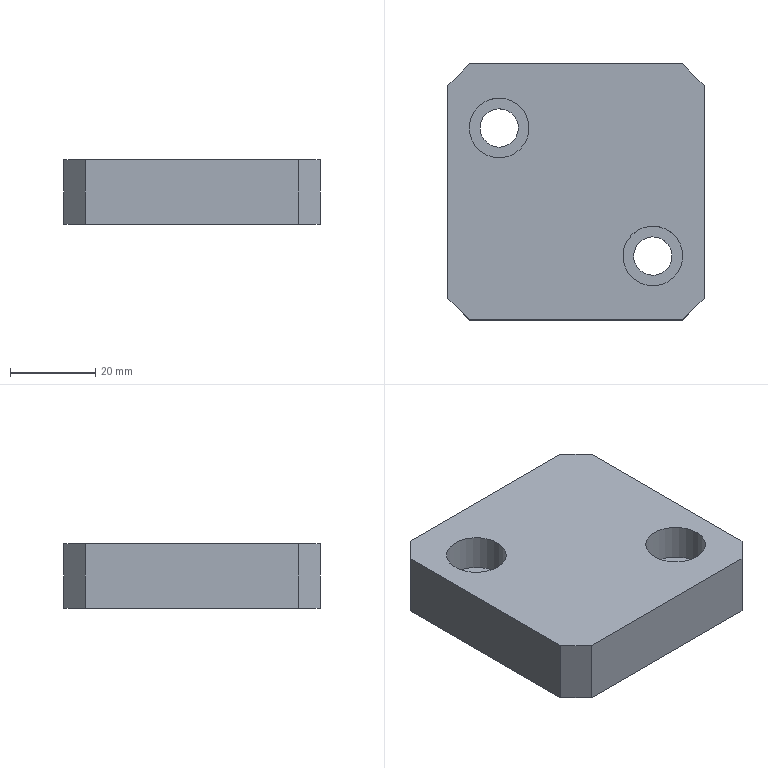Part | NX | features solid 2 | 1 solid | 16 faces | box 60 x 60 x 15 mm | volume 49806 mm3 | plane 12 | cylinder 4 | commonest cylinder face diameters 9 x2 14 x2
STEP:
#1=CARTESIAN_POINT('',(-1130.,-570.,-85.));
#2=VERTEX_POINT('',#1);
#3=CARTESIAN_POINT('',(-1130.,-620.,-85.));
#4=VERTEX_POINT('',#3);
#5=CARTESIAN_POINT('',(-1130.,-545.,-85.));
#6=DIRECTION('',(0.,-1.,0.));
#7=VECTOR('',#6,1000.);
#8=LINE('',#5,#7);
#9=EDGE_CURVE('',#2,#4,#8,.T.);
#10=ORIENTED_EDGE('',*,*,#9,.T.);
#11=CARTESIAN_POINT('',(-1135.,-625.,-85.));
#12=VERTEX_POINT('',#11);
#13=CARTESIAN_POINT('',(-1120.,-610.,-85.));
#14=DIRECTION('',(-0.7071,-0.7071,0.));
#15=VECTOR('',#14,1000.);
#16=LINE('',#13,#15);
#17=EDGE_CURVE('',#12,#4,#16,.F.);
#18=ORIENTED_EDGE('',*,*,#17,.F.);
#19=CARTESIAN_POINT('',(-1185.,-625.,-85.));
#20=VERTEX_POINT('',#19);
#21=CARTESIAN_POINT('',(-1185.,-625.,-85.));
#22=DIRECTION('',(-1.,0.,0.));
#23=VECTOR('',#22,1000.);
#24=LINE('',#21,#23);
#25=EDGE_CURVE('',#20,#12,#24,.F.);
#26=ORIENTED_EDGE('',*,*,#25,.F.);
#27=CARTESIAN_POINT('',(-1190.,-620.,-85.));
#28=VERTEX_POINT('',#27);
#29=CARTESIAN_POINT('',(-1225.,-585.,-85.));
#30=DIRECTION('',(0.7071,-0.7071,0.));
#31=VECTOR('',#30,1000.);
#32=LINE('',#29,#31);
#33=EDGE_CURVE('',#28,#20,#32,.T.);
#34=ORIENTED_EDGE('',*,*,#33,.F.);
#35=CARTESIAN_POINT('',(-1190.,-570.,-85.));
#36=VERTEX_POINT('',#35);
#37=CARTESIAN_POINT('',(-1190.,-553.,-85.));
#38=DIRECTION('',(0.,-1.,0.));
#39=VECTOR('',#38,1000.);
#40=LINE('',#37,#39);
#41=EDGE_CURVE('',#36,#28,#40,.T.);
#42=ORIENTED_EDGE('',*,*,#41,.F.);
#43=CARTESIAN_POINT('',(-1185.,-565.,-85.));
#44=VERTEX_POINT('',#43);
#45=CARTESIAN_POINT('',(-1172.5,-552.5,-85.));
#46=DIRECTION('',(0.7071,0.7071,0.));
#47=VECTOR('',#46,1000.);
#48=LINE('',#45,#47);
#49=EDGE_CURVE('',#44,#36,#48,.F.);
#50=ORIENTED_EDGE('',*,*,#49,.F.);
#51=CARTESIAN_POINT('',(-1135.,-565.,-85.));
#52=VERTEX_POINT('',#51);
#53=CARTESIAN_POINT('',(-1185.,-565.,-85.));
#54=DIRECTION('',(1.,0.,0.));
#55=VECTOR('',#54,1000.);
#56=LINE('',#53,#55);
#57=EDGE_CURVE('',#44,#52,#56,.T.);
#58=ORIENTED_EDGE('',*,*,#57,.T.);
#59=CARTESIAN_POINT('',(-1172.5,-527.5,-85.));
#60=DIRECTION('',(-0.7071,0.7071,0.));
#61=VECTOR('',#60,1000.);
#62=LINE('',#59,#61);
#63=EDGE_CURVE('',#2,#52,#62,.T.);
#64=ORIENTED_EDGE('',*,*,#63,.F.);
#65=EDGE_LOOP('',(#10,#18,#26,#34,#42,#50,#58,#64));
#66=FACE_BOUND('',#65,.T.);
#67=CARTESIAN_POINT('',(-1137.568,-609.219,-85.));
#68=VERTEX_POINT('',#67);
#69=CARTESIAN_POINT('',(-1142.,-610.,-85.));
#70=DIRECTION('',(0.,0.,-1.));
#71=DIRECTION('',(0.9848,0.1736,0.));
#72=AXIS2_PLACEMENT_3D('',#69,#70,#71);
#73=CIRCLE('',#72,4.5);
#74=EDGE_CURVE('',#68,#68,#73,.F.);
#75=ORIENTED_EDGE('',*,*,#74,.T.);
#76=EDGE_LOOP('',(#75));
#77=FACE_BOUND('',#76,.T.);
#78=CARTESIAN_POINT('',(-1173.568,-579.219,-85.));
#79=VERTEX_POINT('',#78);
#80=CARTESIAN_POINT('',(-1178.,-580.,-85.));
#81=DIRECTION('',(0.,0.,-1.));
#82=DIRECTION('',(0.9848,0.1736,0.));
#83=AXIS2_PLACEMENT_3D('',#80,#81,#82);
#84=CIRCLE('',#83,4.5);
#85=EDGE_CURVE('',#79,#79,#84,.F.);
#86=ORIENTED_EDGE('',*,*,#85,.T.);
#87=EDGE_LOOP('',(#86));
#88=FACE_BOUND('',#87,.T.);
#89=CARTESIAN_POINT('',(-1185.,-545.,-85.));
#90=DIRECTION('',(0.,0.,-1.));
#91=DIRECTION('',(1.,0.,0.));
#92=AXIS2_PLACEMENT_3D('',#89,#90,#91);
#93=PLANE('',#92);
#94=ADVANCED_FACE('',(#66,#77,#88),#93,.T.);
#95=CARTESIAN_POINT('',(-1171.106,-578.784,-78.5));
#96=VERTEX_POINT('',#95);
#97=CARTESIAN_POINT('',(-1178.,-580.,-78.5));
#98=DIRECTION('',(0.,0.,-1.));
#99=DIRECTION('',(0.9848,0.1736,0.));
#100=AXIS2_PLACEMENT_3D('',#97,#98,#99);
#101=CIRCLE('',#100,7.);
#102=EDGE_CURVE('',#96,#96,#101,.T.);
#103=ORIENTED_EDGE('',*,*,#102,.F.);
#104=EDGE_LOOP('',(#103));
#105=FACE_BOUND('',#104,.T.);
#106=CARTESIAN_POINT('',(-1173.568,-579.219,-78.5));
#107=VERTEX_POINT('',#106);
#108=CARTESIAN_POINT('',(-1178.,-580.,-78.5));
#109=DIRECTION('',(0.,0.,-1.));
#110=DIRECTION('',(0.9848,0.1736,0.));
#111=AXIS2_PLACEMENT_3D('',#108,#109,#110);
#112=CIRCLE('',#111,4.5);
#113=EDGE_CURVE('',#107,#107,#112,.F.);
#114=ORIENTED_EDGE('',*,*,#113,.F.);
#115=EDGE_LOOP('',(#114));
#116=FACE_BOUND('',#115,.T.);
#117=CARTESIAN_POINT('',(-1185.,-574.5,-78.5));
#118=DIRECTION('',(0.,0.,-1.));
#119=DIRECTION('',(0.9848,0.1736,0.));
#120=AXIS2_PLACEMENT_3D('',#117,#118,#119);
#121=PLANE('',#120);
#122=ADVANCED_FACE('',(#105,#116),#121,.F.);
#123=CARTESIAN_POINT('',(-1185.,-565.,-70.));
#124=VERTEX_POINT('',#123);
#125=CARTESIAN_POINT('',(-1135.,-565.,-70.));
#126=VERTEX_POINT('',#125);
#127=CARTESIAN_POINT('',(-1185.,-565.,-70.));
#128=DIRECTION('',(1.,0.,0.));
#129=VECTOR('',#128,1000.);
#130=LINE('',#127,#129);
#131=EDGE_CURVE('',#124,#126,#130,.T.);
#132=ORIENTED_EDGE('',*,*,#131,.F.);
#133=CARTESIAN_POINT('',(-1190.,-570.,-70.));
#134=VERTEX_POINT('',#133);
#135=CARTESIAN_POINT('',(-1190.,-570.,-70.));
#136=DIRECTION('',(-0.7071,-0.7071,0.));
#137=VECTOR('',#136,1000.);
#138=LINE('',#135,#137);
#139=EDGE_CURVE('',#134,#124,#138,.F.);
#140=ORIENTED_EDGE('',*,*,#139,.F.);
#141=CARTESIAN_POINT('',(-1190.,-620.,-70.));
#142=VERTEX_POINT('',#141);
#143=CARTESIAN_POINT('',(-1190.,-553.,-70.));
#144=DIRECTION('',(0.,-1.,0.));
#145=VECTOR('',#144,1000.);
#146=LINE('',#143,#145);
#147=EDGE_CURVE('',#134,#142,#146,.T.);
#148=ORIENTED_EDGE('',*,*,#147,.T.);
#149=CARTESIAN_POINT('',(-1185.,-625.,-70.));
#150=VERTEX_POINT('',#149);
#151=CARTESIAN_POINT('',(-1190.,-620.,-70.));
#152=DIRECTION('',(-0.7071,0.7071,0.));
#153=VECTOR('',#152,1000.);
#154=LINE('',#151,#153);
#155=EDGE_CURVE('',#150,#142,#154,.T.);
#156=ORIENTED_EDGE('',*,*,#155,.F.);
#157=CARTESIAN_POINT('',(-1135.,-625.,-70.));
#158=VERTEX_POINT('',#157);
#159=CARTESIAN_POINT('',(-1155.,-625.,-70.));
#160=DIRECTION('',(1.,0.,0.));
#161=VECTOR('',#160,1000.);
#162=LINE('',#159,#161);
#163=EDGE_CURVE('',#158,#150,#162,.F.);
#164=ORIENTED_EDGE('',*,*,#163,.F.);
#165=CARTESIAN_POINT('',(-1130.,-620.,-70.));
#166=VERTEX_POINT('',#165);
#167=CARTESIAN_POINT('',(-1130.,-620.,-70.));
#168=DIRECTION('',(0.7071,0.7071,0.));
#169=VECTOR('',#168,1000.);
#170=LINE('',#167,#169);
#171=EDGE_CURVE('',#166,#158,#170,.F.);
#172=ORIENTED_EDGE('',*,*,#171,.F.);
#173=CARTESIAN_POINT('',(-1130.,-570.,-70.));
#174=VERTEX_POINT('',#173);
#175=CARTESIAN_POINT('',(-1130.,-545.,-70.));
#176=DIRECTION('',(0.,-1.,0.));
#177=VECTOR('',#176,1000.);
#178=LINE('',#175,#177);
#179=EDGE_CURVE('',#174,#166,#178,.T.);
#180=ORIENTED_EDGE('',*,*,#179,.F.);
#181=CARTESIAN_POINT('',(-1135.,-565.,-70.));
#182=DIRECTION('',(0.7071,-0.7071,0.));
#183=VECTOR('',#182,1000.);
#184=LINE('',#181,#183);
#185=EDGE_CURVE('',#126,#174,#184,.T.);
#186=ORIENTED_EDGE('',*,*,#185,.F.);
#187=EDGE_LOOP('',(#132,#140,#148,#156,#164,#172,#180,#186));
#188=FACE_BOUND('',#187,.T.);
#189=CARTESIAN_POINT('',(-1135.106,-608.784,-70.));
#190=VERTEX_POINT('',#189);
#191=CARTESIAN_POINT('',(-1142.,-610.,-70.));
#192=DIRECTION('',(0.,0.,-1.));
#193=DIRECTION('',(0.9848,0.1736,0.));
#194=AXIS2_PLACEMENT_3D('',#191,#192,#193);
#195=CIRCLE('',#194,7.);
#196=EDGE_CURVE('',#190,#190,#195,.T.);
#197=ORIENTED_EDGE('',*,*,#196,.T.);
#198=EDGE_LOOP('',(#197));
#199=FACE_BOUND('',#198,.T.);
#200=CARTESIAN_POINT('',(-1171.106,-578.784,-70.));
#201=VERTEX_POINT('',#200);
#202=CARTESIAN_POINT('',(-1178.,-580.,-70.));
#203=DIRECTION('',(0.,0.,-1.));
#204=DIRECTION('',(0.9848,0.1736,0.));
#205=AXIS2_PLACEMENT_3D('',#202,#203,#204);
#206=CIRCLE('',#205,7.);
#207=EDGE_CURVE('',#201,#201,#206,.T.);
#208=ORIENTED_EDGE('',*,*,#207,.T.);
#209=EDGE_LOOP('',(#208));
#210=FACE_BOUND('',#209,.T.);
#211=CARTESIAN_POINT('',(-1185.,-545.,-70.));
#212=DIRECTION('',(0.,0.,-1.));
#213=DIRECTION('',(1.,0.,0.));
#214=AXIS2_PLACEMENT_3D('',#211,#212,#213);
#215=PLANE('',#214);
#216=ADVANCED_FACE('',(#188,#199,#210),#215,.F.);
#217=ORIENTED_EDGE('',*,*,#179,.T.);
#218=CARTESIAN_POINT('',(-1130.,-620.,-70.));
#219=DIRECTION('',(0.,0.,1.));
#220=VECTOR('',#219,1000.);
#221=LINE('',#218,#220);
#222=EDGE_CURVE('',#4,#166,#221,.T.);
#223=ORIENTED_EDGE('',*,*,#222,.F.);
#224=ORIENTED_EDGE('',*,*,#9,.F.);
#225=CARTESIAN_POINT('',(-1130.,-570.,-85.));
#226=DIRECTION('',(0.,0.,-1.));
#227=VECTOR('',#226,1000.);
#228=LINE('',#225,#227);
#229=EDGE_CURVE('',#174,#2,#228,.T.);
#230=ORIENTED_EDGE('',*,*,#229,.F.);
#231=EDGE_LOOP('',(#217,#223,#224,#230));
#232=FACE_BOUND('',#231,.T.);
#233=CARTESIAN_POINT('',(-1130.,-545.,-70.));
#234=DIRECTION('',(1.,0.,0.));
#235=DIRECTION('',(0.,0.,1.));
#236=AXIS2_PLACEMENT_3D('',#233,#234,#235);
#237=PLANE('',#236);
#238=ADVANCED_FACE('',(#232),#237,.T.);
#239=ORIENTED_EDGE('',*,*,#41,.T.);
#240=CARTESIAN_POINT('',(-1190.,-620.,-70.));
#241=DIRECTION('',(0.,0.,-1.));
#242=VECTOR('',#241,1000.);
#243=LINE('',#240,#242);
#244=EDGE_CURVE('',#142,#28,#243,.T.);
#245=ORIENTED_EDGE('',*,*,#244,.F.);
#246=ORIENTED_EDGE('',*,*,#147,.F.);
#247=CARTESIAN_POINT('',(-1190.,-570.,-70.));
#248=DIRECTION('',(0.,0.,1.));
#249=VECTOR('',#248,1000.);
#250=LINE('',#247,#249);
#251=EDGE_CURVE('',#36,#134,#250,.T.);
#252=ORIENTED_EDGE('',*,*,#251,.F.);
#253=EDGE_LOOP('',(#239,#245,#246,#252));
#254=FACE_BOUND('',#253,.T.);
#255=CARTESIAN_POINT('',(-1190.,-553.,-70.));
#256=DIRECTION('',(1.,0.,0.));
#257=DIRECTION('',(0.,1.,0.));
#258=AXIS2_PLACEMENT_3D('',#255,#256,#257);
#259=PLANE('',#258);
#260=ADVANCED_FACE('',(#254),#259,.F.);
#261=ORIENTED_EDGE('',*,*,#25,.T.);
#262=CARTESIAN_POINT('',(-1135.,-625.,-85.));
#263=DIRECTION('',(0.,0.,1.));
#264=VECTOR('',#263,1000.);
#265=LINE('',#262,#264);
#266=EDGE_CURVE('',#158,#12,#265,.F.);
#267=ORIENTED_EDGE('',*,*,#266,.F.);
#268=ORIENTED_EDGE('',*,*,#163,.T.);
#269=CARTESIAN_POINT('',(-1185.,-625.,-70.));
#270=DIRECTION('',(0.,0.,-1.));
#271=VECTOR('',#270,1000.);
#272=LINE('',#269,#271);
#273=EDGE_CURVE('',#20,#150,#272,.F.);
#274=ORIENTED_EDGE('',*,*,#273,.F.);
#275=EDGE_LOOP('',(#261,#267,#268,#274));
#276=FACE_BOUND('',#275,.T.);
#277=CARTESIAN_POINT('',(-1155.,-625.,-70.));
#278=DIRECTION('',(0.,-1.,0.));
#279=DIRECTION('',(0.,0.,1.));
#280=AXIS2_PLACEMENT_3D('',#277,#278,#279);
#281=PLANE('',#280);
#282=ADVANCED_FACE('',(#276),#281,.T.);
#283=ORIENTED_EDGE('',*,*,#196,.F.);
#284=EDGE_LOOP('',(#283));
#285=FACE_BOUND('',#284,.T.);
#286=CARTESIAN_POINT('',(-1135.106,-608.784,-78.5));
#287=VERTEX_POINT('',#286);
#288=CARTESIAN_POINT('',(-1142.,-610.,-78.5));
#289=DIRECTION('',(0.,0.,-1.));
#290=DIRECTION('',(0.9848,0.1736,0.));
#291=AXIS2_PLACEMENT_3D('',#288,#289,#290);
#292=CIRCLE('',#291,7.);
#293=EDGE_CURVE('',#287,#287,#292,.T.);
#294=ORIENTED_EDGE('',*,*,#293,.T.);
#295=EDGE_LOOP('',(#294));
#296=FACE_BOUND('',#295,.T.);
#297=CARTESIAN_POINT('',(-1142.,-610.,-78.5));
#298=DIRECTION('',(0.,0.,1.));
#299=DIRECTION('',(-0.9848,-0.1736,0.));
#300=AXIS2_PLACEMENT_3D('',#297,#298,#299);
#301=CYLINDRICAL_SURFACE('',#300,7.);
#302=ADVANCED_FACE('',(#285,#296),#301,.F.);
#303=CARTESIAN_POINT('',(-1137.568,-609.219,-78.5));
#304=VERTEX_POINT('',#303);
#305=CARTESIAN_POINT('',(-1142.,-610.,-78.5));
#306=DIRECTION('',(0.,0.,-1.));
#307=DIRECTION('',(0.9848,0.1736,0.));
#308=AXIS2_PLACEMENT_3D('',#305,#306,#307);
#309=CIRCLE('',#308,4.5);
#310=EDGE_CURVE('',#304,#304,#309,.F.);
#311=ORIENTED_EDGE('',*,*,#310,.F.);
#312=EDGE_LOOP('',(#311));
#313=FACE_BOUND('',#312,.T.);
#314=ORIENTED_EDGE('',*,*,#293,.F.);
#315=EDGE_LOOP('',(#314));
#316=FACE_BOUND('',#315,.T.);
#317=CARTESIAN_POINT('',(-1145.,-599.5,-78.5));
#318=DIRECTION('',(0.,0.,-1.));
#319=DIRECTION('',(0.9848,0.1736,0.));
#320=AXIS2_PLACEMENT_3D('',#317,#318,#319);
#321=PLANE('',#320);
#322=ADVANCED_FACE('',(#313,#316),#321,.F.);
#323=ORIENTED_EDGE('',*,*,#207,.F.);
#324=EDGE_LOOP('',(#323));
#325=FACE_BOUND('',#324,.T.);
#326=ORIENTED_EDGE('',*,*,#102,.T.);
#327=EDGE_LOOP('',(#326));
#328=FACE_BOUND('',#327,.T.);
#329=CARTESIAN_POINT('',(-1178.,-580.,-78.5));
#330=DIRECTION('',(0.,0.,1.));
#331=DIRECTION('',(-0.9848,-0.1736,0.));
#332=AXIS2_PLACEMENT_3D('',#329,#330,#331);
#333=CYLINDRICAL_SURFACE('',#332,7.);
#334=ADVANCED_FACE('',(#325,#328),#333,.F.);
#335=ORIENTED_EDGE('',*,*,#113,.T.);
#336=EDGE_LOOP('',(#335));
#337=FACE_BOUND('',#336,.T.);
#338=ORIENTED_EDGE('',*,*,#85,.F.);
#339=EDGE_LOOP('',(#338));
#340=FACE_BOUND('',#339,.T.);
#341=CARTESIAN_POINT('',(-1178.,-580.,-170.));
#342=DIRECTION('',(0.,0.,1.));
#343=DIRECTION('',(-0.9848,-0.1736,0.));
#344=AXIS2_PLACEMENT_3D('',#341,#342,#343);
#345=CYLINDRICAL_SURFACE('',#344,4.5);
#346=ADVANCED_FACE('',(#337,#340),#345,.F.);
#347=ORIENTED_EDGE('',*,*,#310,.T.);
#348=EDGE_LOOP('',(#347));
#349=FACE_BOUND('',#348,.T.);
#350=ORIENTED_EDGE('',*,*,#74,.F.);
#351=EDGE_LOOP('',(#350));
#352=FACE_BOUND('',#351,.T.);
#353=CARTESIAN_POINT('',(-1142.,-610.,-170.));
#354=DIRECTION('',(0.,0.,1.));
#355=DIRECTION('',(-0.9848,-0.1736,0.));
#356=AXIS2_PLACEMENT_3D('',#353,#354,#355);
#357=CYLINDRICAL_SURFACE('',#356,4.5);
#358=ADVANCED_FACE('',(#349,#352),#357,.F.);
#359=ORIENTED_EDGE('',*,*,#155,.T.);
#360=ORIENTED_EDGE('',*,*,#244,.T.);
#361=ORIENTED_EDGE('',*,*,#33,.T.);
#362=ORIENTED_EDGE('',*,*,#273,.T.);
#363=EDGE_LOOP('',(#359,#360,#361,#362));
#364=FACE_BOUND('',#363,.T.);
#365=CARTESIAN_POINT('',(-1190.,-620.,-70.));
#366=DIRECTION('',(-0.7071,-0.7071,0.));
#367=DIRECTION('',(-0.7071,0.7071,0.));
#368=AXIS2_PLACEMENT_3D('',#365,#366,#367);
#369=PLANE('',#368);
#370=ADVANCED_FACE('',(#364),#369,.T.);
#371=ORIENTED_EDGE('',*,*,#17,.T.);
#372=ORIENTED_EDGE('',*,*,#222,.T.);
#373=ORIENTED_EDGE('',*,*,#171,.T.);
#374=ORIENTED_EDGE('',*,*,#266,.T.);
#375=EDGE_LOOP('',(#371,#372,#373,#374));
#376=FACE_BOUND('',#375,.T.);
#377=CARTESIAN_POINT('',(-1130.,-620.,-70.));
#378=DIRECTION('',(-0.7071,0.7071,0.));
#379=DIRECTION('',(0.7071,0.7071,0.));
#380=AXIS2_PLACEMENT_3D('',#377,#378,#379);
#381=PLANE('',#380);
#382=ADVANCED_FACE('',(#376),#381,.F.);
#383=ORIENTED_EDGE('',*,*,#57,.F.);
#384=CARTESIAN_POINT('',(-1185.,-565.,-77.5));
#385=DIRECTION('',(0.,0.,-1.));
#386=VECTOR('',#385,1000.);
#387=LINE('',#384,#386);
#388=EDGE_CURVE('',#124,#44,#387,.T.);
#389=ORIENTED_EDGE('',*,*,#388,.F.);
#390=ORIENTED_EDGE('',*,*,#131,.T.);
#391=CARTESIAN_POINT('',(-1135.,-565.,-70.));
#392=DIRECTION('',(0.,0.,1.));
#393=VECTOR('',#392,1000.);
#394=LINE('',#391,#393);
#395=EDGE_CURVE('',#52,#126,#394,.T.);
#396=ORIENTED_EDGE('',*,*,#395,.F.);
#397=EDGE_LOOP('',(#383,#389,#390,#396));
#398=FACE_BOUND('',#397,.T.);
#399=CARTESIAN_POINT('',(-1160.,-565.,-77.5));
#400=DIRECTION('',(0.,-1.,0.));
#401=DIRECTION('',(-1.,0.,0.));
#402=AXIS2_PLACEMENT_3D('',#399,#400,#401);
#403=PLANE('',#402);
#404=ADVANCED_FACE('',(#398),#403,.F.);
#405=ORIENTED_EDGE('',*,*,#63,.T.);
#406=ORIENTED_EDGE('',*,*,#395,.T.);
#407=ORIENTED_EDGE('',*,*,#185,.T.);
#408=ORIENTED_EDGE('',*,*,#229,.T.);
#409=EDGE_LOOP('',(#405,#406,#407,#408));
#410=FACE_BOUND('',#409,.T.);
#411=CARTESIAN_POINT('',(-1135.,-565.,-77.5));
#412=DIRECTION('',(0.7071,0.7071,0.));
#413=DIRECTION('',(0.7071,-0.7071,0.));
#414=AXIS2_PLACEMENT_3D('',#411,#412,#413);
#415=PLANE('',#414);
#416=ADVANCED_FACE('',(#410),#415,.T.);
#417=ORIENTED_EDGE('',*,*,#49,.T.);
#418=ORIENTED_EDGE('',*,*,#251,.T.);
#419=ORIENTED_EDGE('',*,*,#139,.T.);
#420=ORIENTED_EDGE('',*,*,#388,.T.);
#421=EDGE_LOOP('',(#417,#418,#419,#420));
#422=FACE_BOUND('',#421,.T.);
#423=CARTESIAN_POINT('',(-1190.,-570.,-70.));
#424=DIRECTION('',(0.7071,-0.7071,0.));
#425=DIRECTION('',(-0.7071,-0.7071,0.));
#426=AXIS2_PLACEMENT_3D('',#423,#424,#425);
#427=PLANE('',#426);
#428=ADVANCED_FACE('',(#422),#427,.F.);
#429=CLOSED_SHELL('',(#94,#122,#216,#238,#260,#282,#302,#322,#334,#346,#358,#370,#382,#404,#416,#428));
#430=MANIFOLD_SOLID_BREP('',#429);
#431=(LENGTH_UNIT()NAMED_UNIT(*)SI_UNIT(.MILLI.,.METRE.));
#432=UNCERTAINTY_MEASURE_WITH_UNIT(LENGTH_MEASURE(0.00001),#431,'','');
#433=(NAMED_UNIT(*)PLANE_ANGLE_UNIT()SI_UNIT($,.RADIAN.));
#434=(NAMED_UNIT(*)SI_UNIT($,.STERADIAN.)SOLID_ANGLE_UNIT());
#435=(GEOMETRIC_REPRESENTATION_CONTEXT(3)GLOBAL_UNCERTAINTY_ASSIGNED_CONTEXT((#432))GLOBAL_UNIT_ASSIGNED_CONTEXT((#431,#433,#434))REPRESENTATION_CONTEXT('',''));
#436=ADVANCED_BREP_SHAPE_REPRESENTATION('',(#430),#435);